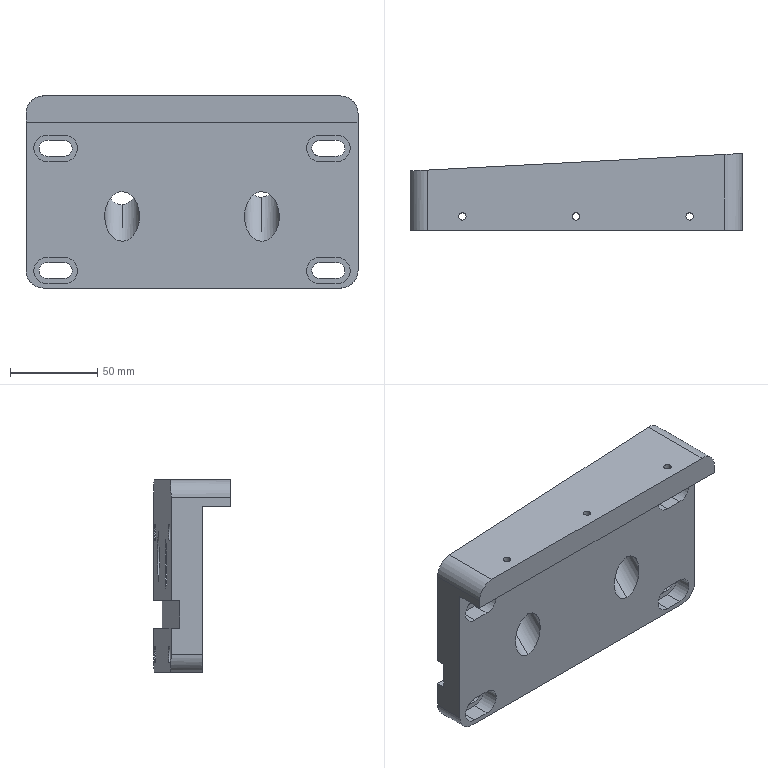Part | SolidWorks | features ICE 4, Extrusion 1, Fillet 1, HoleWzd 1, MirrorPattern 1, SweepCut 1 | 1 solid | 62 faces | box 190 x 44 x 110 mm | volume 466301 mm3 | plane 32 | cylinder 30 | commonest cylinder face diameters 9 x8 15 x8 20 x8 4.2 x6